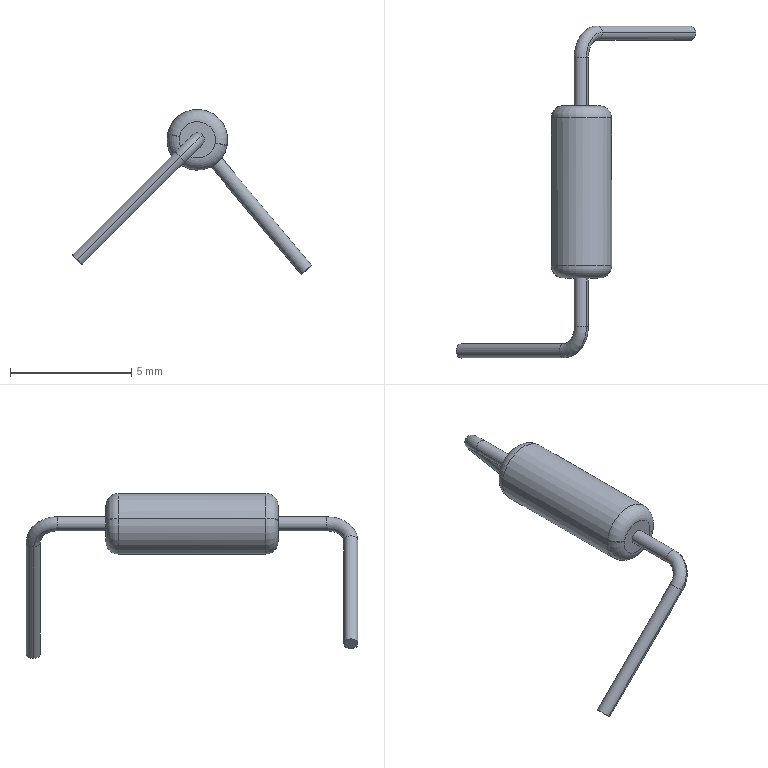Part | SolidWorks | features BaseBody 1 | 1 solid | 27 faces | box 9.876 x 13.68 x 6.803 mm | volume 39.142 mm3 | torus 13 | cylinder 10 | plane 4 | commonest cylinder face diameters 0.58 x8 2.5 x2
STEP:
#1=CARTESIAN_POINT('',(2053.438,-25.555,829.159));
#2=VERTEX_POINT('',#1);
#3=CARTESIAN_POINT('',(2053.419,-25.555,828.732));
#4=VERTEX_POINT('',#3);
#5=CARTESIAN_POINT('',(2053.232,-25.555,828.955));
#6=DIRECTION('',(0.,1.,0.));
#7=DIRECTION('',(0.7079,0.,0.7063));
#8=AXIS2_PLACEMENT_3D('',#5,#6,#7);
#9=CIRCLE('',#8,0.29);
#10=EDGE_CURVE('',#2,#4,#9,.T.);
#11=ORIENTED_EDGE('',*,*,#10,.T.);
#12=CARTESIAN_POINT('',(2053.874,-24.845,828.188));
#13=VERTEX_POINT('',#12);
#14=CARTESIAN_POINT('',(2053.874,-25.555,828.188));
#15=DIRECTION('',(-0.7668,0.,-0.6419));
#16=DIRECTION('',(-0.6419,0.,0.7668));
#17=AXIS2_PLACEMENT_3D('',#14,#15,#16);
#18=CIRCLE('',#17,0.71);
#19=EDGE_CURVE('',#4,#13,#18,.T.);
#20=ORIENTED_EDGE('',*,*,#19,.T.);
#21=CARTESIAN_POINT('',(2054.096,-24.53,828.373));
#22=VERTEX_POINT('',#21);
#23=CARTESIAN_POINT('',(2053.874,-24.555,828.188));
#24=DIRECTION('',(0.6419,0.,-0.7668));
#25=DIRECTION('',(0.7638,0.08716,0.6395));
#26=AXIS2_PLACEMENT_3D('',#23,#24,#25);
#27=CIRCLE('',#26,0.29);
#28=EDGE_CURVE('',#22,#13,#27,.T.);
#29=ORIENTED_EDGE('',*,*,#28,.F.);
#30=CARTESIAN_POINT('',(2053.438,-25.555,829.159));
#31=CARTESIAN_POINT('',(2053.438,-25.478,829.159));
#32=CARTESIAN_POINT('',(2053.449,-25.325,829.146));
#33=CARTESIAN_POINT('',(2053.498,-25.106,829.088));
#34=CARTESIAN_POINT('',(2053.577,-24.91,828.993));
#35=CARTESIAN_POINT('',(2053.682,-24.747,828.868));
#36=CARTESIAN_POINT('',(2053.808,-24.623,828.717));
#37=CARTESIAN_POINT('',(2053.948,-24.547,828.55));
#38=CARTESIAN_POINT('',(2054.047,-24.53,828.432));
#39=CARTESIAN_POINT('',(2054.096,-24.53,828.373));
#40=B_SPLINE_CURVE_WITH_KNOTS('',3,(#30,#31,#32,#33,#34,#35,#36,#37,#38,#39),.UNSPECIFIED.,.F.,.F.,(4,1,1,1,1,1,1,4),(0.,0.1429,0.2857,0.4286,0.5714,0.7143,0.8571,1.),.UNSPECIFIED.);
#41=EDGE_CURVE('',#2,#22,#40,.T.);
#42=ORIENTED_EDGE('',*,*,#41,.F.);
#43=EDGE_LOOP('',(#11,#20,#29,#42));
#44=FACE_OUTER_BOUND('',#43,.T.);
#45=CARTESIAN_POINT('',(2053.874,-25.555,828.188));
#46=DIRECTION('',(-0.7668,0.,-0.6419));
#47=DIRECTION('',(-0.6419,0.,0.7668));
#48=AXIS2_PLACEMENT_3D('',#45,#46,#47);
#49=TOROIDAL_SURFACE('',#48,1.,0.29);
#50=ADVANCED_FACE('',(#44),#49,.T.);
#51=CARTESIAN_POINT('',(2052.002,-28.055,829.173));
#52=VERTEX_POINT('',#51);
#53=CARTESIAN_POINT('',(2054.465,-28.055,828.748));
#54=VERTEX_POINT('',#53);
#55=CARTESIAN_POINT('',(2053.232,-28.055,828.955));
#56=DIRECTION('',(0.,1.,0.));
#57=DIRECTION('',(-0.9846,0.,0.1747));
#58=AXIS2_PLACEMENT_3D('',#55,#56,#57);
#59=CIRCLE('',#58,1.25);
#60=EDGE_CURVE('',#52,#54,#59,.T.);
#61=ORIENTED_EDGE('',*,*,#60,.T.);
#62=CARTESIAN_POINT('',(2053.972,-27.555,828.831));
#63=VERTEX_POINT('',#62);
#64=CARTESIAN_POINT('',(2053.972,-28.055,828.831));
#65=DIRECTION('',(0.1651,0.,0.9863));
#66=DIRECTION('',(0.9863,0.,-0.1651));
#67=AXIS2_PLACEMENT_3D('',#64,#65,#66);
#68=CIRCLE('',#67,0.5);
#69=EDGE_CURVE('',#54,#63,#68,.T.);
#70=ORIENTED_EDGE('',*,*,#69,.T.);
#71=CARTESIAN_POINT('',(2052.494,-27.555,829.086));
#72=VERTEX_POINT('',#71);
#73=CARTESIAN_POINT('',(2053.232,-27.555,828.955));
#74=DIRECTION('',(0.,1.,0.));
#75=DIRECTION('',(-0.9846,0.,0.1747));
#76=AXIS2_PLACEMENT_3D('',#73,#74,#75);
#77=CIRCLE('',#76,0.75);
#78=EDGE_CURVE('',#72,#63,#77,.T.);
#79=ORIENTED_EDGE('',*,*,#78,.F.);
#80=CARTESIAN_POINT('',(2052.494,-28.055,829.086));
#81=DIRECTION('',(-0.1747,0.,-0.9846));
#82=DIRECTION('',(0.,1.,0.));
#83=AXIS2_PLACEMENT_3D('',#80,#81,#82);
#84=CIRCLE('',#83,0.5);
#85=EDGE_CURVE('',#52,#72,#84,.T.);
#86=ORIENTED_EDGE('',*,*,#85,.F.);
#87=EDGE_LOOP('',(#61,#70,#79,#86));
#88=FACE_OUTER_BOUND('',#87,.T.);
#89=CARTESIAN_POINT('',(2053.232,-28.055,828.955));
#90=DIRECTION('',(0.,1.,0.));
#91=DIRECTION('',(0.9863,0.,-0.1651));
#92=AXIS2_PLACEMENT_3D('',#89,#90,#91);
#93=TOROIDAL_SURFACE('',#92,0.75,0.5);
#94=ADVANCED_FACE('',(#88),#93,.T.);
#95=CARTESIAN_POINT('',(2054.463,-28.055,828.736));
#96=VERTEX_POINT('',#95);
#97=CARTESIAN_POINT('',(2052.,-28.055,829.161));
#98=VERTEX_POINT('',#97);
#99=CARTESIAN_POINT('',(2053.232,-28.055,828.955));
#100=DIRECTION('',(0.,1.,0.));
#101=DIRECTION('',(0.9846,0.,-0.1747));
#102=AXIS2_PLACEMENT_3D('',#99,#100,#101);
#103=CIRCLE('',#102,1.25);
#104=EDGE_CURVE('',#96,#98,#103,.T.);
#105=ORIENTED_EDGE('',*,*,#104,.T.);
#106=CARTESIAN_POINT('',(2052.493,-27.555,829.079));
#107=VERTEX_POINT('',#106);
#108=CARTESIAN_POINT('',(2052.493,-28.055,829.079));
#109=DIRECTION('',(-0.1651,0.,-0.9863));
#110=DIRECTION('',(-0.9863,0.,0.1651));
#111=AXIS2_PLACEMENT_3D('',#108,#109,#110);
#112=CIRCLE('',#111,0.5);
#113=EDGE_CURVE('',#98,#107,#112,.T.);
#114=ORIENTED_EDGE('',*,*,#113,.T.);
#115=CARTESIAN_POINT('',(2053.971,-27.555,828.824));
#116=VERTEX_POINT('',#115);
#117=CARTESIAN_POINT('',(2053.232,-27.555,828.955));
#118=DIRECTION('',(0.,1.,0.));
#119=DIRECTION('',(0.9846,0.,-0.1747));
#120=AXIS2_PLACEMENT_3D('',#117,#118,#119);
#121=CIRCLE('',#120,0.75);
#122=EDGE_CURVE('',#116,#107,#121,.T.);
#123=ORIENTED_EDGE('',*,*,#122,.F.);
#124=CARTESIAN_POINT('',(2053.971,-28.055,828.824));
#125=DIRECTION('',(-0.1747,0.,-0.9846));
#126=DIRECTION('',(0.,1.,0.));
#127=AXIS2_PLACEMENT_3D('',#124,#125,#126);
#128=CIRCLE('',#127,0.5);
#129=EDGE_CURVE('',#116,#96,#128,.T.);
#130=ORIENTED_EDGE('',*,*,#129,.T.);
#131=EDGE_LOOP('',(#105,#114,#123,#130));
#132=FACE_OUTER_BOUND('',#131,.T.);
#133=CARTESIAN_POINT('',(2053.232,-28.055,828.955));
#134=DIRECTION('',(0.,1.,0.));
#135=DIRECTION('',(-0.9863,0.,0.1651));
#136=AXIS2_PLACEMENT_3D('',#133,#134,#135);
#137=TOROIDAL_SURFACE('',#136,0.75,0.5);
#138=ADVANCED_FACE('',(#132),#137,.T.);
#139=CARTESIAN_POINT('',(2053.969,-34.655,828.813));
#140=VERTEX_POINT('',#139);
#141=CARTESIAN_POINT('',(2053.971,-34.655,828.824));
#142=VERTEX_POINT('',#141);
#143=CARTESIAN_POINT('',(2053.232,-34.655,828.955));
#144=DIRECTION('',(0.,-1.,0.));
#145=DIRECTION('',(-0.9846,0.,0.1747));
#146=AXIS2_PLACEMENT_3D('',#143,#144,#145);
#147=CIRCLE('',#146,0.75);
#148=EDGE_CURVE('',#140,#142,#147,.T.);
#149=ORIENTED_EDGE('',*,*,#148,.F.);
#150=CARTESIAN_POINT('',(2054.46,-34.155,828.719));
#151=VERTEX_POINT('',#150);
#152=CARTESIAN_POINT('',(2053.969,-34.155,828.813));
#153=DIRECTION('',(0.1884,0.,0.9821));
#154=DIRECTION('',(0.9821,0.,-0.1884));
#155=AXIS2_PLACEMENT_3D('',#152,#153,#154);
#156=CIRCLE('',#155,0.5);
#157=EDGE_CURVE('',#140,#151,#156,.T.);
#158=ORIENTED_EDGE('',*,*,#157,.T.);
#159=CARTESIAN_POINT('',(2054.463,-34.155,828.736));
#160=VERTEX_POINT('',#159);
#161=CARTESIAN_POINT('',(2053.232,-34.155,828.955));
#162=DIRECTION('',(0.,-1.,0.));
#163=DIRECTION('',(-0.9846,0.,0.1747));
#164=AXIS2_PLACEMENT_3D('',#161,#162,#163);
#165=CIRCLE('',#164,1.25);
#166=EDGE_CURVE('',#151,#160,#165,.T.);
#167=ORIENTED_EDGE('',*,*,#166,.T.);
#168=CARTESIAN_POINT('',(2053.971,-34.155,828.824));
#169=DIRECTION('',(0.1747,0.,0.9846));
#170=DIRECTION('',(0.,-1.,0.));
#171=AXIS2_PLACEMENT_3D('',#168,#169,#170);
#172=CIRCLE('',#171,0.5);
#173=EDGE_CURVE('',#142,#160,#172,.T.);
#174=ORIENTED_EDGE('',*,*,#173,.F.);
#175=EDGE_LOOP('',(#149,#158,#167,#174));
#176=FACE_OUTER_BOUND('',#175,.T.);
#177=CARTESIAN_POINT('',(2053.232,-34.155,828.955));
#178=DIRECTION('',(0.,1.,0.));
#179=DIRECTION('',(0.9821,0.,-0.1884));
#180=AXIS2_PLACEMENT_3D('',#177,#178,#179);
#181=TOROIDAL_SURFACE('',#180,0.75,0.5);
#182=ADVANCED_FACE('',(#176),#181,.T.);
#183=CARTESIAN_POINT('',(2052.496,-34.655,829.096));
#184=VERTEX_POINT('',#183);
#185=CARTESIAN_POINT('',(2052.494,-34.655,829.086));
#186=VERTEX_POINT('',#185);
#187=CARTESIAN_POINT('',(2053.232,-34.655,828.955));
#188=DIRECTION('',(0.,-1.,0.));
#189=DIRECTION('',(0.9846,0.,-0.1747));
#190=AXIS2_PLACEMENT_3D('',#187,#188,#189);
#191=CIRCLE('',#190,0.75);
#192=EDGE_CURVE('',#184,#186,#191,.T.);
#193=ORIENTED_EDGE('',*,*,#192,.F.);
#194=CARTESIAN_POINT('',(2052.005,-34.155,829.19));
#195=VERTEX_POINT('',#194);
#196=CARTESIAN_POINT('',(2052.496,-34.155,829.096));
#197=DIRECTION('',(-0.1884,0.,-0.9821));
#198=DIRECTION('',(-0.9821,0.,0.1884));
#199=AXIS2_PLACEMENT_3D('',#196,#197,#198);
#200=CIRCLE('',#199,0.5);
#201=EDGE_CURVE('',#184,#195,#200,.T.);
#202=ORIENTED_EDGE('',*,*,#201,.T.);
#203=CARTESIAN_POINT('',(2052.002,-34.155,829.173));
#204=VERTEX_POINT('',#203);
#205=CARTESIAN_POINT('',(2053.232,-34.155,828.955));
#206=DIRECTION('',(0.,-1.,0.));
#207=DIRECTION('',(0.9846,0.,-0.1747));
#208=AXIS2_PLACEMENT_3D('',#205,#206,#207);
#209=CIRCLE('',#208,1.25);
#210=EDGE_CURVE('',#195,#204,#209,.T.);
#211=ORIENTED_EDGE('',*,*,#210,.T.);
#212=CARTESIAN_POINT('',(2052.494,-34.155,829.086));
#213=DIRECTION('',(0.1747,0.,0.9846));
#214=DIRECTION('',(0.,-1.,0.));
#215=AXIS2_PLACEMENT_3D('',#212,#213,#214);
#216=CIRCLE('',#215,0.5);
#217=EDGE_CURVE('',#204,#186,#216,.T.);
#218=ORIENTED_EDGE('',*,*,#217,.T.);
#219=EDGE_LOOP('',(#193,#202,#211,#218));
#220=FACE_OUTER_BOUND('',#219,.T.);
#221=CARTESIAN_POINT('',(2053.232,-34.155,828.955));
#222=DIRECTION('',(0.,1.,0.));
#223=DIRECTION('',(-0.9821,0.,0.1884));
#224=AXIS2_PLACEMENT_3D('',#221,#222,#223);
#225=TOROIDAL_SURFACE('',#224,0.75,0.5);
#226=ADVANCED_FACE('',(#220),#225,.T.);
#227=CARTESIAN_POINT('',(2053.232,-34.655,828.955));
#228=DIRECTION('',(0.,-1.,0.));
#229=DIRECTION('',(-0.9846,0.,0.1747));
#230=AXIS2_PLACEMENT_3D('',#227,#228,#229);
#231=CIRCLE('',#230,0.75);
#232=EDGE_CURVE('',#186,#140,#231,.T.);
#233=ORIENTED_EDGE('',*,*,#232,.T.);
#234=ORIENTED_EDGE('',*,*,#148,.T.);
#235=CARTESIAN_POINT('',(2053.232,-34.655,828.955));
#236=DIRECTION('',(0.,-1.,0.));
#237=DIRECTION('',(0.9846,0.,-0.1747));
#238=AXIS2_PLACEMENT_3D('',#235,#236,#237);
#239=CIRCLE('',#238,0.75);
#240=EDGE_CURVE('',#142,#184,#239,.T.);
#241=ORIENTED_EDGE('',*,*,#240,.T.);
#242=ORIENTED_EDGE('',*,*,#192,.T.);
#243=EDGE_LOOP('',(#233,#234,#241,#242));
#244=FACE_OUTER_BOUND('',#243,.T.);
#245=CARTESIAN_POINT('',(2053.438,-34.655,829.159));
#246=VERTEX_POINT('',#245);
#247=CARTESIAN_POINT('',(2053.027,-34.655,828.75));
#248=VERTEX_POINT('',#247);
#249=CARTESIAN_POINT('',(2053.232,-34.655,828.955));
#250=DIRECTION('',(0.,1.,0.));
#251=DIRECTION('',(0.7079,0.,0.7063));
#252=AXIS2_PLACEMENT_3D('',#249,#250,#251);
#253=CIRCLE('',#252,0.29);
#254=EDGE_CURVE('',#246,#248,#253,.T.);
#255=ORIENTED_EDGE('',*,*,#254,.T.);
#256=CARTESIAN_POINT('',(2053.232,-34.655,828.955));
#257=DIRECTION('',(0.,1.,0.));
#258=DIRECTION('',(-0.7079,0.,-0.7063));
#259=AXIS2_PLACEMENT_3D('',#256,#257,#258);
#260=CIRCLE('',#259,0.29);
#261=EDGE_CURVE('',#248,#246,#260,.T.);
#262=ORIENTED_EDGE('',*,*,#261,.T.);
#263=EDGE_LOOP('',(#255,#262));
#264=FACE_BOUND('',#263,.T.);
#265=CARTESIAN_POINT('',(2053.232,-34.655,828.955));
#266=DIRECTION('',(0.,1.,0.));
#267=DIRECTION('',(0.9846,0.,-0.1747));
#268=AXIS2_PLACEMENT_3D('',#265,#266,#267);
#269=PLANE('',#268);
#270=ADVANCED_FACE('',(#244,#264),#269,.F.);
#271=ORIENTED_EDGE('',*,*,#201,.F.);
#272=ORIENTED_EDGE('',*,*,#240,.F.);
#273=ORIENTED_EDGE('',*,*,#173,.T.);
#274=CARTESIAN_POINT('',(2053.232,-34.155,828.955));
#275=DIRECTION('',(0.,-1.,0.));
#276=DIRECTION('',(0.9846,0.,-0.1747));
#277=AXIS2_PLACEMENT_3D('',#274,#275,#276);
#278=CIRCLE('',#277,1.25);
#279=EDGE_CURVE('',#160,#195,#278,.T.);
#280=ORIENTED_EDGE('',*,*,#279,.T.);
#281=EDGE_LOOP('',(#271,#272,#273,#280));
#282=FACE_OUTER_BOUND('',#281,.T.);
#283=CARTESIAN_POINT('',(2053.232,-34.155,828.955));
#284=DIRECTION('',(0.,1.,0.));
#285=DIRECTION('',(-0.9821,0.,0.1884));
#286=AXIS2_PLACEMENT_3D('',#283,#284,#285);
#287=TOROIDAL_SURFACE('',#286,0.75,0.5);
#288=ADVANCED_FACE('',(#282),#287,.T.);
#289=ORIENTED_EDGE('',*,*,#157,.F.);
#290=ORIENTED_EDGE('',*,*,#232,.F.);
#291=ORIENTED_EDGE('',*,*,#217,.F.);
#292=CARTESIAN_POINT('',(2053.232,-34.155,828.955));
#293=DIRECTION('',(0.,-1.,0.));
#294=DIRECTION('',(-0.9846,0.,0.1747));
#295=AXIS2_PLACEMENT_3D('',#292,#293,#294);
#296=CIRCLE('',#295,1.25);
#297=EDGE_CURVE('',#204,#151,#296,.T.);
#298=ORIENTED_EDGE('',*,*,#297,.T.);
#299=EDGE_LOOP('',(#289,#290,#291,#298));
#300=FACE_OUTER_BOUND('',#299,.T.);
#301=CARTESIAN_POINT('',(2053.232,-34.155,828.955));
#302=DIRECTION('',(0.,1.,0.));
#303=DIRECTION('',(0.9821,0.,-0.1884));
#304=AXIS2_PLACEMENT_3D('',#301,#302,#303);
#305=TOROIDAL_SURFACE('',#304,0.75,0.5);
#306=ADVANCED_FACE('',(#300),#305,.T.);
#307=CARTESIAN_POINT('',(2054.463,-34.155,828.736));
#308=DIRECTION('',(0.,-1.,0.));
#309=VECTOR('',#308,1000.);
#310=LINE('',#307,#309);
#311=EDGE_CURVE('',#96,#160,#310,.T.);
#312=ORIENTED_EDGE('',*,*,#311,.T.);
#313=ORIENTED_EDGE('',*,*,#166,.F.);
#314=ORIENTED_EDGE('',*,*,#297,.F.);
#315=CARTESIAN_POINT('',(2052.002,-34.155,829.173));
#316=DIRECTION('',(0.,1.,0.));
#317=VECTOR('',#316,1000.);
#318=LINE('',#315,#317);
#319=EDGE_CURVE('',#204,#52,#318,.T.);
#320=ORIENTED_EDGE('',*,*,#319,.T.);
#321=CARTESIAN_POINT('',(2053.232,-28.055,828.955));
#322=DIRECTION('',(0.,1.,0.));
#323=DIRECTION('',(0.9846,0.,-0.1747));
#324=AXIS2_PLACEMENT_3D('',#321,#322,#323);
#325=CIRCLE('',#324,1.25);
#326=EDGE_CURVE('',#98,#52,#325,.T.);
#327=ORIENTED_EDGE('',*,*,#326,.F.);
#328=ORIENTED_EDGE('',*,*,#104,.F.);
#329=EDGE_LOOP('',(#312,#313,#314,#320,#327,#328));
#330=FACE_OUTER_BOUND('',#329,.T.);
#331=CARTESIAN_POINT('',(2053.232,-34.655,828.955));
#332=DIRECTION('',(0.,1.,0.));
#333=DIRECTION('',(0.9846,0.,-0.1747));
#334=AXIS2_PLACEMENT_3D('',#331,#332,#333);
#335=CYLINDRICAL_SURFACE('',#334,1.25);
#336=ADVANCED_FACE('',(#330),#335,.T.);
#337=ORIENTED_EDGE('',*,*,#113,.F.);
#338=ORIENTED_EDGE('',*,*,#326,.T.);
#339=ORIENTED_EDGE('',*,*,#85,.T.);
#340=CARTESIAN_POINT('',(2053.232,-27.555,828.955));
#341=DIRECTION('',(0.,1.,0.));
#342=DIRECTION('',(0.9846,0.,-0.1747));
#343=AXIS2_PLACEMENT_3D('',#340,#341,#342);
#344=CIRCLE('',#343,0.75);
#345=EDGE_CURVE('',#107,#72,#344,.T.);
#346=ORIENTED_EDGE('',*,*,#345,.F.);
#347=EDGE_LOOP('',(#337,#338,#339,#346));
#348=FACE_OUTER_BOUND('',#347,.T.);
#349=CARTESIAN_POINT('',(2053.232,-28.055,828.955));
#350=DIRECTION('',(0.,1.,0.));
#351=DIRECTION('',(-0.9863,0.,0.1651));
#352=AXIS2_PLACEMENT_3D('',#349,#350,#351);
#353=TOROIDAL_SURFACE('',#352,0.75,0.5);
#354=ADVANCED_FACE('',(#348),#353,.T.);
#355=ORIENTED_EDGE('',*,*,#78,.T.);
#356=CARTESIAN_POINT('',(2053.232,-27.555,828.955));
#357=DIRECTION('',(0.,1.,0.));
#358=DIRECTION('',(-0.9846,0.,0.1747));
#359=AXIS2_PLACEMENT_3D('',#356,#357,#358);
#360=CIRCLE('',#359,0.75);
#361=EDGE_CURVE('',#63,#116,#360,.T.);
#362=ORIENTED_EDGE('',*,*,#361,.T.);
#363=ORIENTED_EDGE('',*,*,#122,.T.);
#364=ORIENTED_EDGE('',*,*,#345,.T.);
#365=EDGE_LOOP('',(#355,#362,#363,#364));
#366=FACE_OUTER_BOUND('',#365,.T.);
#367=CARTESIAN_POINT('',(2053.438,-27.555,829.159));
#368=VERTEX_POINT('',#367);
#369=CARTESIAN_POINT('',(2053.027,-27.555,828.75));
#370=VERTEX_POINT('',#369);
#371=CARTESIAN_POINT('',(2053.232,-27.555,828.955));
#372=DIRECTION('',(0.,1.,0.));
#373=DIRECTION('',(0.7079,0.,0.7063));
#374=AXIS2_PLACEMENT_3D('',#371,#372,#373);
#375=CIRCLE('',#374,0.29);
#376=EDGE_CURVE('',#368,#370,#375,.T.);
#377=ORIENTED_EDGE('',*,*,#376,.F.);
#378=CARTESIAN_POINT('',(2053.232,-27.555,828.955));
#379=DIRECTION('',(0.,1.,0.));
#380=DIRECTION('',(-0.7079,0.,-0.7063));
#381=AXIS2_PLACEMENT_3D('',#378,#379,#380);
#382=CIRCLE('',#381,0.29);
#383=EDGE_CURVE('',#370,#368,#382,.T.);
#384=ORIENTED_EDGE('',*,*,#383,.F.);
#385=EDGE_LOOP('',(#377,#384));
#386=FACE_BOUND('',#385,.T.);
#387=CARTESIAN_POINT('',(2053.232,-27.555,828.955));
#388=DIRECTION('',(0.,1.,0.));
#389=DIRECTION('',(0.9846,0.,-0.1747));
#390=AXIS2_PLACEMENT_3D('',#387,#388,#389);
#391=PLANE('',#390);
#392=ADVANCED_FACE('',(#366,#386),#391,.T.);
#393=ORIENTED_EDGE('',*,*,#69,.F.);
#394=CARTESIAN_POINT('',(2053.232,-28.055,828.955));
#395=DIRECTION('',(0.,1.,0.));
#396=DIRECTION('',(-0.9846,0.,0.1747));
#397=AXIS2_PLACEMENT_3D('',#394,#395,#396);
#398=CIRCLE('',#397,1.25);
#399=EDGE_CURVE('',#54,#96,#398,.T.);
#400=ORIENTED_EDGE('',*,*,#399,.T.);
#401=ORIENTED_EDGE('',*,*,#129,.F.);
#402=ORIENTED_EDGE('',*,*,#361,.F.);
#403=EDGE_LOOP('',(#393,#400,#401,#402));
#404=FACE_OUTER_BOUND('',#403,.T.);
#405=CARTESIAN_POINT('',(2053.232,-28.055,828.955));
#406=DIRECTION('',(0.,1.,0.));
#407=DIRECTION('',(0.9863,0.,-0.1651));
#408=AXIS2_PLACEMENT_3D('',#405,#406,#407);
#409=TOROIDAL_SURFACE('',#408,0.75,0.5);
#410=ADVANCED_FACE('',(#404),#409,.T.);
#411=ORIENTED_EDGE('',*,*,#319,.F.);
#412=ORIENTED_EDGE('',*,*,#210,.F.);
#413=ORIENTED_EDGE('',*,*,#279,.F.);
#414=ORIENTED_EDGE('',*,*,#311,.F.);
#415=ORIENTED_EDGE('',*,*,#399,.F.);
#416=ORIENTED_EDGE('',*,*,#60,.F.);
#417=EDGE_LOOP('',(#411,#412,#413,#414,#415,#416));
#418=FACE_OUTER_BOUND('',#417,.T.);
#419=CARTESIAN_POINT('',(2053.232,-34.655,828.955));
#420=DIRECTION('',(0.,1.,0.));
#421=DIRECTION('',(0.9846,0.,-0.1747));
#422=AXIS2_PLACEMENT_3D('',#419,#420,#421);
#423=CYLINDRICAL_SURFACE('',#422,1.25);
#424=ADVANCED_FACE('',(#418),#423,.T.);
#425=CARTESIAN_POINT('',(2053.438,-27.555,829.159));
#426=DIRECTION('',(0.,-1.,0.));
#427=VECTOR('',#426,1000.);
#428=LINE('',#425,#427);
#429=EDGE_CURVE('',#2,#368,#428,.T.);
#430=ORIENTED_EDGE('',*,*,#429,.F.);
#431=CARTESIAN_POINT('',(2053.027,-25.555,828.75));
#432=VERTEX_POINT('',#431);
#433=CARTESIAN_POINT('',(2053.232,-25.555,828.955));
#434=DIRECTION('',(0.,1.,0.));
#435=DIRECTION('',(-0.7079,0.,-0.7063));
#436=AXIS2_PLACEMENT_3D('',#433,#434,#435);
#437=CIRCLE('',#436,0.29);
#438=EDGE_CURVE('',#432,#2,#437,.T.);
#439=ORIENTED_EDGE('',*,*,#438,.F.);
#440=CARTESIAN_POINT('',(2053.027,-27.555,828.75));
#441=DIRECTION('',(0.,1.,0.));
#442=VECTOR('',#441,1000.);
#443=LINE('',#440,#442);
#444=EDGE_CURVE('',#370,#432,#443,.T.);
#445=ORIENTED_EDGE('',*,*,#444,.F.);
#446=ORIENTED_EDGE('',*,*,#383,.T.);
#447=EDGE_LOOP('',(#430,#439,#445,#446));
#448=FACE_OUTER_BOUND('',#447,.T.);
#449=CARTESIAN_POINT('',(2053.232,-31.105,828.955));
#450=DIRECTION('',(0.,1.,0.));
#451=DIRECTION('',(0.7079,0.,0.7063));
#452=AXIS2_PLACEMENT_3D('',#449,#450,#451);
#453=CYLINDRICAL_SURFACE('',#452,0.29);
#454=ADVANCED_FACE('',(#448),#453,.T.);
#455=ORIENTED_EDGE('',*,*,#444,.T.);
#456=CARTESIAN_POINT('',(2053.232,-25.555,828.955));
#457=DIRECTION('',(0.,1.,0.));
#458=DIRECTION('',(0.7079,0.,0.7063));
#459=AXIS2_PLACEMENT_3D('',#456,#457,#458);
#460=CIRCLE('',#459,0.29);
#461=EDGE_CURVE('',#4,#432,#460,.T.);
#462=ORIENTED_EDGE('',*,*,#461,.F.);
#463=ORIENTED_EDGE('',*,*,#10,.F.);
#464=ORIENTED_EDGE('',*,*,#429,.T.);
#465=ORIENTED_EDGE('',*,*,#376,.T.);
#466=EDGE_LOOP('',(#455,#462,#463,#464,#465));
#467=FACE_OUTER_BOUND('',#466,.T.);
#468=CARTESIAN_POINT('',(2053.232,-31.105,828.955));
#469=DIRECTION('',(0.,1.,0.));
#470=DIRECTION('',(0.7079,0.,0.7063));
#471=AXIS2_PLACEMENT_3D('',#468,#469,#470);
#472=CYLINDRICAL_SURFACE('',#471,0.29);
#473=ADVANCED_FACE('',(#467),#472,.T.);
#474=ORIENTED_EDGE('',*,*,#19,.F.);
#475=ORIENTED_EDGE('',*,*,#461,.T.);
#476=CARTESIAN_POINT('',(2053.653,-24.58,828.002));
#477=VERTEX_POINT('',#476);
#478=CARTESIAN_POINT('',(2053.653,-24.58,828.002));
#479=CARTESIAN_POINT('',(2053.606,-24.58,828.058));
#480=CARTESIAN_POINT('',(2053.512,-24.597,828.17));
#481=CARTESIAN_POINT('',(2053.379,-24.669,828.329));
#482=CARTESIAN_POINT('',(2053.259,-24.787,828.472));
#483=CARTESIAN_POINT('',(2053.16,-24.942,828.592));
#484=CARTESIAN_POINT('',(2053.084,-25.129,828.681));
#485=CARTESIAN_POINT('',(2053.038,-25.336,828.737));
#486=CARTESIAN_POINT('',(2053.027,-25.482,828.75));
#487=CARTESIAN_POINT('',(2053.027,-25.555,828.75));
#488=B_SPLINE_CURVE_WITH_KNOTS('',3,(#478,#479,#480,#481,#482,#483,#484,#485,#486,#487),.UNSPECIFIED.,.F.,.F.,(4,1,1,1,1,1,1,4),(0.,0.1429,0.2857,0.4286,0.5714,0.7143,0.8571,1.),.UNSPECIFIED.);
#489=EDGE_CURVE('',#477,#432,#488,.T.);
#490=ORIENTED_EDGE('',*,*,#489,.F.);
#491=CARTESIAN_POINT('',(2053.874,-24.555,828.188));
#492=DIRECTION('',(0.6419,0.,-0.7668));
#493=DIRECTION('',(0.7638,0.08716,0.6395));
#494=AXIS2_PLACEMENT_3D('',#491,#492,#493);
#495=CIRCLE('',#494,0.29);
#496=EDGE_CURVE('',#13,#477,#495,.T.);
#497=ORIENTED_EDGE('',*,*,#496,.F.);
#498=EDGE_LOOP('',(#474,#475,#490,#497));
#499=FACE_OUTER_BOUND('',#498,.T.);
#500=CARTESIAN_POINT('',(2053.874,-25.555,828.188));
#501=DIRECTION('',(-0.7668,0.,-0.6419));
#502=DIRECTION('',(-0.6419,0.,0.7668));
#503=AXIS2_PLACEMENT_3D('',#500,#501,#502);
#504=TOROIDAL_SURFACE('',#503,1.,0.29);
#505=ADVANCED_FACE('',(#499),#504,.T.);
#506=ORIENTED_EDGE('',*,*,#41,.T.);
#507=CARTESIAN_POINT('',(2053.874,-24.555,828.188));
#508=DIRECTION('',(0.6419,0.,-0.7668));
#509=DIRECTION('',(-0.7638,-0.08716,-0.6395));
#510=AXIS2_PLACEMENT_3D('',#507,#508,#509);
#511=CIRCLE('',#510,0.29);
#512=EDGE_CURVE('',#477,#22,#511,.T.);
#513=ORIENTED_EDGE('',*,*,#512,.F.);
#514=ORIENTED_EDGE('',*,*,#489,.T.);
#515=ORIENTED_EDGE('',*,*,#438,.T.);
#516=EDGE_LOOP('',(#506,#513,#514,#515));
#517=FACE_OUTER_BOUND('',#516,.T.);
#518=CARTESIAN_POINT('',(2053.874,-25.555,828.188));
#519=DIRECTION('',(-0.7668,0.,-0.6419));
#520=DIRECTION('',(-0.6419,0.,0.7668));
#521=AXIS2_PLACEMENT_3D('',#518,#519,#520);
#522=TOROIDAL_SURFACE('',#521,1.,0.29);
#523=ADVANCED_FACE('',(#517),#522,.T.);
#524=CARTESIAN_POINT('',(2057.948,-24.53,823.773));
#525=VERTEX_POINT('',#524);
#526=CARTESIAN_POINT('',(2054.096,-24.53,828.373));
#527=DIRECTION('',(-0.6419,0.,0.7668));
#528=VECTOR('',#527,1000.);
#529=LINE('',#526,#528);
#530=EDGE_CURVE('',#525,#22,#529,.T.);
#531=ORIENTED_EDGE('',*,*,#530,.F.);
#532=CARTESIAN_POINT('',(2057.504,-24.58,823.402));
#533=VERTEX_POINT('',#532);
#534=CARTESIAN_POINT('',(2057.726,-24.555,823.587));
#535=DIRECTION('',(0.6419,0.,-0.7668));
#536=DIRECTION('',(-0.7638,-0.08716,-0.6395));
#537=AXIS2_PLACEMENT_3D('',#534,#535,#536);
#538=CIRCLE('',#537,0.29);
#539=EDGE_CURVE('',#533,#525,#538,.T.);
#540=ORIENTED_EDGE('',*,*,#539,.F.);
#541=CARTESIAN_POINT('',(2053.653,-24.58,828.002));
#542=DIRECTION('',(0.6419,0.,-0.7668));
#543=VECTOR('',#542,1000.);
#544=LINE('',#541,#543);
#545=EDGE_CURVE('',#477,#533,#544,.T.);
#546=ORIENTED_EDGE('',*,*,#545,.F.);
#547=ORIENTED_EDGE('',*,*,#512,.T.);
#548=EDGE_LOOP('',(#531,#540,#546,#547));
#549=FACE_OUTER_BOUND('',#548,.T.);
#550=CARTESIAN_POINT('',(2053.874,-24.555,828.188));
#551=DIRECTION('',(0.6419,0.,-0.7668));
#552=DIRECTION('',(0.7638,0.08716,0.6395));
#553=AXIS2_PLACEMENT_3D('',#550,#551,#552);
#554=CYLINDRICAL_SURFACE('',#553,0.29);
#555=ADVANCED_FACE('',(#549),#554,.T.);
#556=ORIENTED_EDGE('',*,*,#545,.T.);
#557=CARTESIAN_POINT('',(2057.726,-24.555,823.587));
#558=DIRECTION('',(0.6419,0.,-0.7668));
#559=DIRECTION('',(0.7638,0.08716,0.6395));
#560=AXIS2_PLACEMENT_3D('',#557,#558,#559);
#561=CIRCLE('',#560,0.29);
#562=EDGE_CURVE('',#525,#533,#561,.T.);
#563=ORIENTED_EDGE('',*,*,#562,.F.);
#564=ORIENTED_EDGE('',*,*,#530,.T.);
#565=ORIENTED_EDGE('',*,*,#28,.T.);
#566=ORIENTED_EDGE('',*,*,#496,.T.);
#567=EDGE_LOOP('',(#556,#563,#564,#565,#566));
#568=FACE_OUTER_BOUND('',#567,.T.);
#569=CARTESIAN_POINT('',(2053.874,-24.555,828.188));
#570=DIRECTION('',(0.6419,0.,-0.7668));
#571=DIRECTION('',(0.7638,0.08716,0.6395));
#572=AXIS2_PLACEMENT_3D('',#569,#570,#571);
#573=CYLINDRICAL_SURFACE('',#572,0.29);
#574=ADVANCED_FACE('',(#568),#573,.T.);
#575=ORIENTED_EDGE('',*,*,#562,.T.);
#576=ORIENTED_EDGE('',*,*,#539,.T.);
#577=EDGE_LOOP('',(#575,#576));
#578=FACE_OUTER_BOUND('',#577,.T.);
#579=CARTESIAN_POINT('',(2057.726,-24.555,823.587));
#580=DIRECTION('',(0.6419,0.,-0.7668));
#581=DIRECTION('',(0.7638,0.08716,0.6395));
#582=AXIS2_PLACEMENT_3D('',#579,#580,#581);
#583=PLANE('',#582);
#584=ADVANCED_FACE('',(#578),#583,.T.);
#585=CARTESIAN_POINT('',(2053.027,-36.655,828.75));
#586=VERTEX_POINT('',#585);
#587=CARTESIAN_POINT('',(2053.027,-36.655,828.75));
#588=DIRECTION('',(0.,1.,0.));
#589=VECTOR('',#588,1000.);
#590=LINE('',#587,#589);
#591=EDGE_CURVE('',#586,#248,#590,.T.);
#592=ORIENTED_EDGE('',*,*,#591,.F.);
#593=CARTESIAN_POINT('',(2053.438,-36.655,829.159));
#594=VERTEX_POINT('',#593);
#595=CARTESIAN_POINT('',(2053.232,-36.655,828.955));
#596=DIRECTION('',(0.,1.,0.));
#597=DIRECTION('',(-0.7079,0.,-0.7063));
#598=AXIS2_PLACEMENT_3D('',#595,#596,#597);
#599=CIRCLE('',#598,0.29);
#600=EDGE_CURVE('',#586,#594,#599,.T.);
#601=ORIENTED_EDGE('',*,*,#600,.T.);
#602=CARTESIAN_POINT('',(2053.438,-36.655,829.159));
#603=DIRECTION('',(0.,-1.,0.));
#604=VECTOR('',#603,1000.);
#605=LINE('',#602,#604);
#606=EDGE_CURVE('',#246,#594,#605,.T.);
#607=ORIENTED_EDGE('',*,*,#606,.F.);
#608=ORIENTED_EDGE('',*,*,#261,.F.);
#609=EDGE_LOOP('',(#592,#601,#607,#608));
#610=FACE_OUTER_BOUND('',#609,.T.);
#611=CARTESIAN_POINT('',(2053.232,-36.655,828.955));
#612=DIRECTION('',(0.,1.,0.));
#613=DIRECTION('',(0.7079,0.,0.7063));
#614=AXIS2_PLACEMENT_3D('',#611,#612,#613);
#615=CYLINDRICAL_SURFACE('',#614,0.29);
#616=ADVANCED_FACE('',(#610),#615,.T.);
#617=ORIENTED_EDGE('',*,*,#606,.T.);
#618=CARTESIAN_POINT('',(2053.232,-36.655,828.955));
#619=DIRECTION('',(0.,1.,0.));
#620=DIRECTION('',(0.7079,0.,0.7063));
#621=AXIS2_PLACEMENT_3D('',#618,#619,#620);
#622=CIRCLE('',#621,0.29);
#623=EDGE_CURVE('',#594,#586,#622,.T.);
#624=ORIENTED_EDGE('',*,*,#623,.T.);
#625=ORIENTED_EDGE('',*,*,#591,.T.);
#626=ORIENTED_EDGE('',*,*,#254,.F.);
#627=EDGE_LOOP('',(#617,#624,#625,#626));
#628=FACE_OUTER_BOUND('',#627,.T.);
#629=CARTESIAN_POINT('',(2053.232,-36.655,828.955));
#630=DIRECTION('',(0.,1.,0.));
#631=DIRECTION('',(0.7079,0.,0.7063));
#632=AXIS2_PLACEMENT_3D('',#629,#630,#631);
#633=CYLINDRICAL_SURFACE('',#632,0.29);
#634=ADVANCED_FACE('',(#628),#633,.T.);
#635=CARTESIAN_POINT('',(2052.525,-37.365,828.248));
#636=VERTEX_POINT('',#635);
#637=CARTESIAN_POINT('',(2053.027,-36.655,828.75));
#638=CARTESIAN_POINT('',(2053.027,-36.717,828.75));
#639=CARTESIAN_POINT('',(2053.016,-36.841,828.738));
#640=CARTESIAN_POINT('',(2052.965,-37.014,828.688));
#641=CARTESIAN_POINT('',(2052.884,-37.163,828.607));
#642=CARTESIAN_POINT('',(2052.779,-37.277,828.502));
#643=CARTESIAN_POINT('',(2052.656,-37.349,828.38));
#644=CARTESIAN_POINT('',(2052.568,-37.365,828.292));
#645=CARTESIAN_POINT('',(2052.525,-37.365,828.248));
#646=B_SPLINE_CURVE_WITH_KNOTS('',3,(#637,#638,#639,#640,#641,#642,#643,#644,#645),.UNSPECIFIED.,.F.,.F.,(4,1,1,1,1,1,4),(0.,0.1667,0.3333,0.5,0.6667,0.8333,1.),.UNSPECIFIED.);
#647=EDGE_CURVE('',#586,#636,#646,.T.);
#648=ORIENTED_EDGE('',*,*,#647,.F.);
#649=ORIENTED_EDGE('',*,*,#623,.F.);
#650=CARTESIAN_POINT('',(2052.525,-37.945,828.248));
#651=VERTEX_POINT('',#650);
#652=CARTESIAN_POINT('',(2052.525,-37.945,828.248));
#653=CARTESIAN_POINT('',(2052.593,-37.945,828.316));
#654=CARTESIAN_POINT('',(2052.73,-37.923,828.453));
#655=CARTESIAN_POINT('',(2052.924,-37.827,828.647));
#656=CARTESIAN_POINT('',(2053.099,-37.672,828.821));
#657=CARTESIAN_POINT('',(2053.245,-37.466,828.967));
#658=CARTESIAN_POINT('',(2053.354,-37.219,829.076));
#659=CARTESIAN_POINT('',(2053.422,-36.944,829.144));
#660=CARTESIAN_POINT('',(2053.438,-36.751,829.159));
#661=CARTESIAN_POINT('',(2053.438,-36.655,829.159));
#662=B_SPLINE_CURVE_WITH_KNOTS('',3,(#652,#653,#654,#655,#656,#657,#658,#659,#660,#661),.UNSPECIFIED.,.F.,.F.,(4,1,1,1,1,1,1,4),(0.,0.1429,0.2857,0.4286,0.5714,0.7143,0.8571,1.),.UNSPECIFIED.);
#663=EDGE_CURVE('',#651,#594,#662,.T.);
#664=ORIENTED_EDGE('',*,*,#663,.F.);
#665=CARTESIAN_POINT('',(2052.525,-37.655,828.248));
#666=DIRECTION('',(0.7079,0.,0.7063));
#667=DIRECTION('',(0.,-1.,0.));
#668=AXIS2_PLACEMENT_3D('',#665,#666,#667);
#669=CIRCLE('',#668,0.29);
#670=EDGE_CURVE('',#651,#636,#669,.T.);
#671=ORIENTED_EDGE('',*,*,#670,.T.);
#672=EDGE_LOOP('',(#648,#649,#664,#671));
#673=FACE_OUTER_BOUND('',#672,.T.);
#674=CARTESIAN_POINT('',(2052.525,-36.655,828.248));
#675=DIRECTION('',(-0.7063,0.,0.7079));
#676=DIRECTION('',(0.,-1.,0.));
#677=AXIS2_PLACEMENT_3D('',#674,#675,#676);
#678=TOROIDAL_SURFACE('',#677,1.,0.29);
#679=ADVANCED_FACE('',(#673),#678,.T.);
#680=CARTESIAN_POINT('',(2048.277,-37.365,824.01));
#681=VERTEX_POINT('',#680);
#682=CARTESIAN_POINT('',(2048.277,-37.365,824.01));
#683=DIRECTION('',(-0.7079,0.,-0.7063));
#684=VECTOR('',#683,1000.);
#685=LINE('',#682,#684);
#686=EDGE_CURVE('',#636,#681,#685,.T.);
#687=ORIENTED_EDGE('',*,*,#686,.F.);
#688=ORIENTED_EDGE('',*,*,#670,.F.);
#689=CARTESIAN_POINT('',(2048.277,-37.945,824.01));
#690=VERTEX_POINT('',#689);
#691=CARTESIAN_POINT('',(2048.277,-37.945,824.01));
#692=DIRECTION('',(0.7079,0.,0.7063));
#693=VECTOR('',#692,1000.);
#694=LINE('',#691,#693);
#695=EDGE_CURVE('',#690,#651,#694,.T.);
#696=ORIENTED_EDGE('',*,*,#695,.F.);
#697=CARTESIAN_POINT('',(2048.277,-37.655,824.01));
#698=DIRECTION('',(0.7079,0.,0.7063));
#699=DIRECTION('',(0.,-1.,0.));
#700=AXIS2_PLACEMENT_3D('',#697,#698,#699);
#701=CIRCLE('',#700,0.29);
#702=EDGE_CURVE('',#690,#681,#701,.T.);
#703=ORIENTED_EDGE('',*,*,#702,.T.);
#704=EDGE_LOOP('',(#687,#688,#696,#703));
#705=FACE_OUTER_BOUND('',#704,.T.);
#706=CARTESIAN_POINT('',(2048.277,-37.655,824.01));
#707=DIRECTION('',(0.7079,0.,0.7063));
#708=DIRECTION('',(0.,-1.,0.));
#709=AXIS2_PLACEMENT_3D('',#706,#707,#708);
#710=CYLINDRICAL_SURFACE('',#709,0.29);
#711=ADVANCED_FACE('',(#705),#710,.T.);
#712=ORIENTED_EDGE('',*,*,#702,.F.);
#713=CARTESIAN_POINT('',(2048.277,-37.655,824.01));
#714=DIRECTION('',(0.7079,0.,0.7063));
#715=DIRECTION('',(0.,1.,0.));
#716=AXIS2_PLACEMENT_3D('',#713,#714,#715);
#717=CIRCLE('',#716,0.29);
#718=EDGE_CURVE('',#681,#690,#717,.T.);
#719=ORIENTED_EDGE('',*,*,#718,.F.);
#720=EDGE_LOOP('',(#712,#719));
#721=FACE_OUTER_BOUND('',#720,.T.);
#722=CARTESIAN_POINT('',(2048.277,-37.655,824.01));
#723=DIRECTION('',(0.7079,0.,0.7063));
#724=DIRECTION('',(0.,-1.,0.));
#725=AXIS2_PLACEMENT_3D('',#722,#723,#724);
#726=PLANE('',#725);
#727=ADVANCED_FACE('',(#721),#726,.F.);
#728=ORIENTED_EDGE('',*,*,#695,.T.);
#729=CARTESIAN_POINT('',(2052.525,-37.655,828.248));
#730=DIRECTION('',(0.7079,0.,0.7063));
#731=DIRECTION('',(0.,1.,0.));
#732=AXIS2_PLACEMENT_3D('',#729,#730,#731);
#733=CIRCLE('',#732,0.29);
#734=EDGE_CURVE('',#636,#651,#733,.T.);
#735=ORIENTED_EDGE('',*,*,#734,.F.);
#736=ORIENTED_EDGE('',*,*,#686,.T.);
#737=ORIENTED_EDGE('',*,*,#718,.T.);
#738=EDGE_LOOP('',(#728,#735,#736,#737));
#739=FACE_OUTER_BOUND('',#738,.T.);
#740=CARTESIAN_POINT('',(2048.277,-37.655,824.01));
#741=DIRECTION('',(0.7079,0.,0.7063));
#742=DIRECTION('',(0.,-1.,0.));
#743=AXIS2_PLACEMENT_3D('',#740,#741,#742);
#744=CYLINDRICAL_SURFACE('',#743,0.29);
#745=ADVANCED_FACE('',(#739),#744,.T.);
#746=ORIENTED_EDGE('',*,*,#663,.T.);
#747=ORIENTED_EDGE('',*,*,#600,.F.);
#748=ORIENTED_EDGE('',*,*,#647,.T.);
#749=ORIENTED_EDGE('',*,*,#734,.T.);
#750=EDGE_LOOP('',(#746,#747,#748,#749));
#751=FACE_OUTER_BOUND('',#750,.T.);
#752=CARTESIAN_POINT('',(2052.525,-36.655,828.248));
#753=DIRECTION('',(-0.7063,0.,0.7079));
#754=DIRECTION('',(0.,-1.,0.));
#755=AXIS2_PLACEMENT_3D('',#752,#753,#754);
#756=TOROIDAL_SURFACE('',#755,1.,0.29);
#757=ADVANCED_FACE('',(#751),#756,.T.);
#758=CLOSED_SHELL('',(#50,#94,#138,#182,#226,#270,#288,#306,#336,#354,#392,#410,#424,#454,#473,#505,#523,#555,#574,#584,#616,#634,#679,#711,#727,#745,#757));
#759=MANIFOLD_SOLID_BREP('',#758);
#760=CARTESIAN_POINT('',(0.,0.,0.));
#761=DIRECTION('',(0.,0.,1.));
#762=DIRECTION('',(1.,0.,0.));
#763=AXIS2_PLACEMENT_3D('',#760,#761,#762);
#764=(LENGTH_UNIT()NAMED_UNIT(*)SI_UNIT(.MILLI.,.METRE.));
#765=UNCERTAINTY_MEASURE_WITH_UNIT(LENGTH_MEASURE(0.00001),#764,'','');
#766=(NAMED_UNIT(*)PLANE_ANGLE_UNIT()SI_UNIT($,.RADIAN.));
#767=(NAMED_UNIT(*)SI_UNIT($,.STERADIAN.)SOLID_ANGLE_UNIT());
#768=(GEOMETRIC_REPRESENTATION_CONTEXT(3)GLOBAL_UNCERTAINTY_ASSIGNED_CONTEXT((#765))GLOBAL_UNIT_ASSIGNED_CONTEXT((#764,#766,#767))REPRESENTATION_CONTEXT('',''));
#769=ADVANCED_BREP_SHAPE_REPRESENTATION('',(#759,#763),#768);